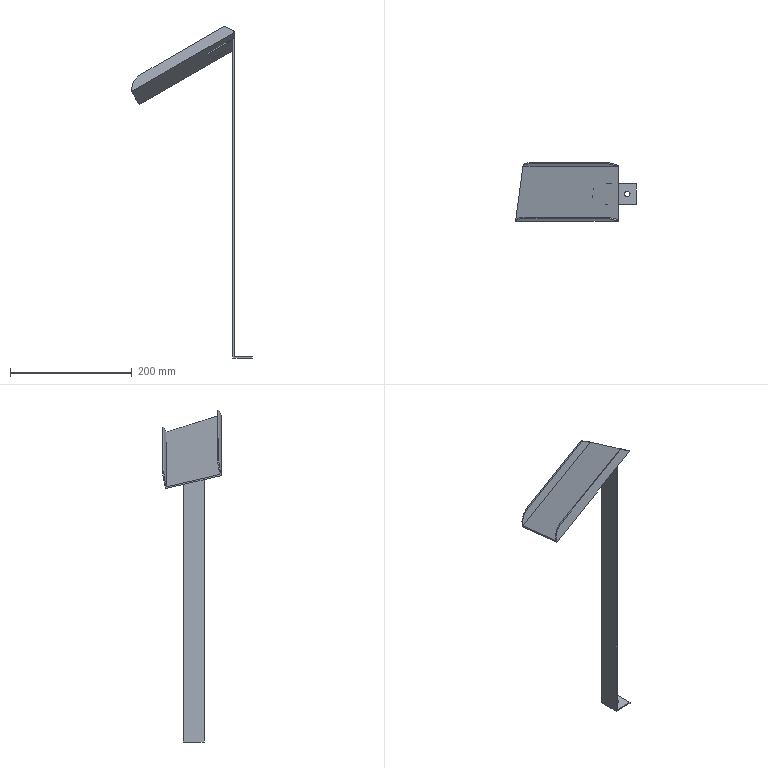Part | NX | features solid 2 | 1 solid | 27 faces | box 198.257 x 96.321 x 544.886 mm | volume 86995 mm3 | plane 24 | cylinder 3 | commonest cylinder face diameters 60 x2 9 x1
STEP:
#1=CARTESIAN_POINT('',(-340.,82.105,-151.35));
#2=VERTEX_POINT('',#1);
#3=CARTESIAN_POINT('',(-383.223,82.105,-176.304));
#4=VERTEX_POINT('',#3);
#5=CARTESIAN_POINT('',(-341.705,82.105,-152.334));
#6=DIRECTION('',(0.866,0.,0.5));
#7=VECTOR('',#6,1000.);
#8=LINE('',#5,#7);
#9=EDGE_CURVE('',#2,#4,#8,.F.);
#10=ORIENTED_EDGE('',*,*,#9,.F.);
#11=CARTESIAN_POINT('',(-340.,55.747,-143.195));
#12=VERTEX_POINT('',#11);
#13=CARTESIAN_POINT('',(-340.,-1199.843,245.286));
#14=DIRECTION('',(0.,0.9553,-0.2956));
#15=VECTOR('',#14,1000.);
#16=LINE('',#13,#15);
#17=EDGE_CURVE('',#12,#2,#16,.T.);
#18=ORIENTED_EDGE('',*,*,#17,.F.);
#19=CARTESIAN_POINT('',(-339.741,55.747,-143.045));
#20=VERTEX_POINT('',#19);
#21=CARTESIAN_POINT('',(-339.741,55.747,-143.045));
#22=DIRECTION('',(-0.866,0.,-0.5));
#23=VECTOR('',#22,1000.);
#24=LINE('',#21,#23);
#25=EDGE_CURVE('',#20,#12,#24,.T.);
#26=ORIENTED_EDGE('',*,*,#25,.F.);
#27=CARTESIAN_POINT('',(-340.,53.815,-142.597));
#28=VERTEX_POINT('',#27);
#29=CARTESIAN_POINT('',(-339.741,55.747,-143.045));
#30=DIRECTION('',(0.1294,0.9659,-0.2241));
#31=VECTOR('',#30,1000.);
#32=LINE('',#29,#31);
#33=EDGE_CURVE('',#20,#28,#32,.F.);
#34=ORIENTED_EDGE('',*,*,#33,.T.);
#35=CARTESIAN_POINT('',(-508.257,53.815,-239.74));
#36=VERTEX_POINT('',#35);
#37=CARTESIAN_POINT('',(-958.517,53.815,-499.698));
#38=DIRECTION('',(-0.866,0.,-0.5));
#39=VECTOR('',#38,1000.);
#40=LINE('',#37,#39);
#41=EDGE_CURVE('',#28,#36,#40,.T.);
#42=ORIENTED_EDGE('',*,*,#41,.T.);
#43=CARTESIAN_POINT('',(-495.958,145.615,-261.042));
#44=VERTEX_POINT('',#43);
#45=CARTESIAN_POINT('',(-693.776,-1330.922,81.59));
#46=DIRECTION('',(-0.1294,-0.9659,0.2241));
#47=VECTOR('',#46,1000.);
#48=LINE('',#45,#47);
#49=EDGE_CURVE('',#36,#44,#48,.F.);
#50=ORIENTED_EDGE('',*,*,#49,.T.);
#51=CARTESIAN_POINT('',(-340.,145.615,-171.));
#52=VERTEX_POINT('',#51);
#53=CARTESIAN_POINT('',(-946.218,145.615,-521.));
#54=DIRECTION('',(-0.866,0.,-0.5));
#55=VECTOR('',#54,1000.);
#56=LINE('',#53,#55);
#57=EDGE_CURVE('',#52,#44,#56,.T.);
#58=ORIENTED_EDGE('',*,*,#57,.F.);
#59=CARTESIAN_POINT('',(-340.,116.29,-161.927));
#60=VERTEX_POINT('',#59);
#61=CARTESIAN_POINT('',(-340.,-1199.843,245.286));
#62=DIRECTION('',(0.,0.9553,-0.2956));
#63=VECTOR('',#62,1000.);
#64=LINE('',#61,#63);
#65=EDGE_CURVE('',#60,#52,#64,.T.);
#66=ORIENTED_EDGE('',*,*,#65,.F.);
#67=CARTESIAN_POINT('',(-378.643,116.29,-184.237));
#68=VERTEX_POINT('',#67);
#69=CARTESIAN_POINT('',(-950.147,116.29,-514.195));
#70=DIRECTION('',(-0.866,0.,-0.5));
#71=VECTOR('',#70,1000.);
#72=LINE('',#69,#71);
#73=EDGE_CURVE('',#60,#68,#72,.T.);
#74=ORIENTED_EDGE('',*,*,#73,.T.);
#75=CARTESIAN_POINT('',(-572.533,-1330.922,151.59));
#76=DIRECTION('',(0.1294,0.9659,-0.2241));
#77=VECTOR('',#76,1000.);
#78=LINE('',#75,#77);
#79=EDGE_CURVE('',#4,#68,#78,.T.);
#80=ORIENTED_EDGE('',*,*,#79,.F.);
#81=EDGE_LOOP('',(#10,#18,#26,#34,#42,#50,#58,#66,#74,#80));
#82=FACE_BOUND('',#81,.T.);
#83=CARTESIAN_POINT('',(-1144.036,-1330.922,-178.368));
#84=DIRECTION('',(-0.483,0.2588,0.8365));
#85=DIRECTION('',(0.866,0.,0.5));
#86=AXIS2_PLACEMENT_3D('',#83,#84,#85);
#87=PLANE('',#86);
#88=ADVANCED_FACE('',(#82),#87,.F.);
#89=CARTESIAN_POINT('',(-340.,56.264,-140.964));
#90=VERTEX_POINT('',#89);
#91=CARTESIAN_POINT('',(-507.998,56.264,-237.957));
#92=VERTEX_POINT('',#91);
#93=CARTESIAN_POINT('',(-959.224,56.264,-498.473));
#94=DIRECTION('',(-0.866,0.,-0.5));
#95=VECTOR('',#94,1000.);
#96=LINE('',#93,#95);
#97=EDGE_CURVE('',#90,#92,#96,.T.);
#98=ORIENTED_EDGE('',*,*,#97,.F.);
#99=CARTESIAN_POINT('',(-340.,146.133,-168.769));
#100=VERTEX_POINT('',#99);
#101=CARTESIAN_POINT('',(-340.,-1199.168,247.468));
#102=DIRECTION('',(0.,0.9553,-0.2956));
#103=VECTOR('',#102,1000.);
#104=LINE('',#101,#103);
#105=EDGE_CURVE('',#90,#100,#104,.T.);
#106=ORIENTED_EDGE('',*,*,#105,.T.);
#107=CARTESIAN_POINT('',(-340.251,146.133,-168.914));
#108=VERTEX_POINT('',#107);
#109=CARTESIAN_POINT('',(-947.184,146.133,-519.327));
#110=DIRECTION('',(-0.866,0.,-0.5));
#111=VECTOR('',#110,1000.);
#112=LINE('',#109,#111);
#113=EDGE_CURVE('',#100,#108,#112,.T.);
#114=ORIENTED_EDGE('',*,*,#113,.T.);
#115=CARTESIAN_POINT('',(-340.51,144.201,-168.466));
#116=VERTEX_POINT('',#115);
#117=CARTESIAN_POINT('',(-538.07,-1330.404,173.717));
#118=DIRECTION('',(-0.1294,-0.9659,0.2241));
#119=VECTOR('',#118,1000.);
#120=LINE('',#117,#119);
#121=EDGE_CURVE('',#116,#108,#120,.F.);
#122=ORIENTED_EDGE('',*,*,#121,.F.);
#123=CARTESIAN_POINT('',(-496.216,144.201,-258.363));
#124=VERTEX_POINT('',#123);
#125=CARTESIAN_POINT('',(-947.443,144.201,-518.879));
#126=DIRECTION('',(-0.866,0.,-0.5));
#127=VECTOR('',#126,1000.);
#128=LINE('',#125,#127);
#129=EDGE_CURVE('',#116,#124,#128,.T.);
#130=ORIENTED_EDGE('',*,*,#129,.T.);
#131=CARTESIAN_POINT('',(-693.776,-1330.404,83.82));
#132=DIRECTION('',(-0.1294,-0.9659,0.2241));
#133=VECTOR('',#132,1000.);
#134=LINE('',#131,#133);
#135=EDGE_CURVE('',#92,#124,#134,.F.);
#136=ORIENTED_EDGE('',*,*,#135,.F.);
#137=EDGE_LOOP('',(#98,#106,#114,#122,#130,#136));
#138=FACE_BOUND('',#137,.T.);
#139=CARTESIAN_POINT('',(-1145.002,-1330.404,-176.695));
#140=DIRECTION('',(-0.483,0.2588,0.8365));
#141=DIRECTION('',(0.866,0.,0.5));
#142=AXIS2_PLACEMENT_3D('',#139,#140,#141);
#143=PLANE('',#142);
#144=ADVANCED_FACE('',(#138),#143,.T.);
#145=CARTESIAN_POINT('',(-340.,11.781,-332.662));
#146=DIRECTION('',(0.,0.226,0.9741));
#147=VECTOR('',#146,1000.);
#148=LINE('',#145,#147);
#149=EDGE_CURVE('',#12,#90,#148,.T.);
#150=ORIENTED_EDGE('',*,*,#149,.F.);
#151=ORIENTED_EDGE('',*,*,#17,.T.);
#152=CARTESIAN_POINT('',(-340.,82.105,-675.));
#153=VERTEX_POINT('',#152);
#154=CARTESIAN_POINT('',(-340.,82.105,-9.));
#155=DIRECTION('',(0.,0.,1.));
#156=VECTOR('',#155,1000.);
#157=LINE('',#154,#156);
#158=EDGE_CURVE('',#2,#153,#157,.F.);
#159=ORIENTED_EDGE('',*,*,#158,.T.);
#160=CARTESIAN_POINT('',(-340.,116.29,-675.));
#161=VERTEX_POINT('',#160);
#162=CARTESIAN_POINT('',(-340.,-710.,-675.));
#163=DIRECTION('',(0.,-1.,0.));
#164=VECTOR('',#163,1000.);
#165=LINE('',#162,#164);
#166=EDGE_CURVE('',#153,#161,#165,.F.);
#167=ORIENTED_EDGE('',*,*,#166,.T.);
#168=CARTESIAN_POINT('',(-340.,116.29,-163.531));
#169=VERTEX_POINT('',#168);
#170=CARTESIAN_POINT('',(-340.,116.29,-9.));
#171=DIRECTION('',(0.,0.,1.));
#172=VECTOR('',#171,1000.);
#173=LINE('',#170,#172);
#174=EDGE_CURVE('',#169,#161,#173,.F.);
#175=ORIENTED_EDGE('',*,*,#174,.F.);
#176=CARTESIAN_POINT('',(-340.,116.29,-9.));
#177=DIRECTION('',(0.,0.,1.));
#178=VECTOR('',#177,1000.);
#179=LINE('',#176,#178);
#180=EDGE_CURVE('',#60,#169,#179,.F.);
#181=ORIENTED_EDGE('',*,*,#180,.F.);
#182=ORIENTED_EDGE('',*,*,#65,.T.);
#183=CARTESIAN_POINT('',(-340.,103.18,-353.871));
#184=DIRECTION('',(0.,0.226,0.9741));
#185=VECTOR('',#184,1000.);
#186=LINE('',#183,#185);
#187=EDGE_CURVE('',#52,#100,#186,.T.);
#188=ORIENTED_EDGE('',*,*,#187,.T.);
#189=ORIENTED_EDGE('',*,*,#105,.F.);
#190=EDGE_LOOP('',(#150,#151,#159,#167,#175,#181,#182,#188,#189));
#191=FACE_BOUND('',#190,.T.);
#192=CARTESIAN_POINT('',(-340.,-1383.009,-9.));
#193=DIRECTION('',(1.,0.,0.));
#194=DIRECTION('',(0.,0.,-1.));
#195=AXIS2_PLACEMENT_3D('',#192,#193,#194);
#196=PLANE('',#195);
#197=ADVANCED_FACE('',(#191),#196,.T.);
#198=CARTESIAN_POINT('',(-340.251,54.333,-140.511));
#199=VERTEX_POINT('',#198);
#200=CARTESIAN_POINT('',(-340.,56.207,-140.946));
#201=VERTEX_POINT('',#200);
#202=CARTESIAN_POINT('',(-525.771,-1330.404,180.818));
#203=DIRECTION('',(-0.1294,-0.9659,0.2241));
#204=VECTOR('',#203,1000.);
#205=LINE('',#202,#204);
#206=EDGE_CURVE('',#199,#201,#205,.F.);
#207=ORIENTED_EDGE('',*,*,#206,.F.);
#208=CARTESIAN_POINT('',(-340.,54.333,-140.366));
#209=VERTEX_POINT('',#208);
#210=CARTESIAN_POINT('',(-959.483,54.333,-498.025));
#211=DIRECTION('',(-0.866,0.,-0.5));
#212=VECTOR('',#211,1000.);
#213=LINE('',#210,#212);
#214=EDGE_CURVE('',#209,#199,#213,.T.);
#215=ORIENTED_EDGE('',*,*,#214,.F.);
#216=CARTESIAN_POINT('',(-340.,-1199.168,247.468));
#217=DIRECTION('',(0.,0.9553,-0.2956));
#218=VECTOR('',#217,1000.);
#219=LINE('',#216,#218);
#220=EDGE_CURVE('',#209,#201,#219,.T.);
#221=ORIENTED_EDGE('',*,*,#220,.T.);
#222=EDGE_LOOP('',(#207,#215,#221));
#223=FACE_BOUND('',#222,.T.);
#224=CARTESIAN_POINT('',(-1145.002,-1330.404,-176.695));
#225=DIRECTION('',(-0.483,0.2588,0.8365));
#226=DIRECTION('',(0.866,0.,0.5));
#227=AXIS2_PLACEMENT_3D('',#224,#225,#226);
#228=PLANE('',#227);
#229=ADVANCED_FACE('',(#223),#228,.T.);
#230=CARTESIAN_POINT('',(-495.958,146.154,-258.723));
#231=VERTEX_POINT('',#230);
#232=CARTESIAN_POINT('',(-495.958,145.868,-259.956));
#233=DIRECTION('',(0.,-0.226,-0.9741));
#234=VECTOR('',#233,1000.);
#235=LINE('',#232,#234);
#236=EDGE_CURVE('',#44,#231,#235,.F.);
#237=ORIENTED_EDGE('',*,*,#236,.F.);
#238=ORIENTED_EDGE('',*,*,#49,.F.);
#239=CARTESIAN_POINT('',(-508.257,54.353,-237.421));
#240=VERTEX_POINT('',#239);
#241=CARTESIAN_POINT('',(-508.257,54.067,-238.653));
#242=DIRECTION('',(0.,-0.226,-0.9741));
#243=VECTOR('',#242,1000.);
#244=LINE('',#241,#243);
#245=EDGE_CURVE('',#36,#240,#244,.F.);
#246=ORIENTED_EDGE('',*,*,#245,.T.);
#247=CARTESIAN_POINT('',(-507.998,56.285,-237.869));
#248=VERTEX_POINT('',#247);
#249=CARTESIAN_POINT('',(-495.958,146.154,-258.723));
#250=DIRECTION('',(-0.1294,-0.9659,0.2241));
#251=VECTOR('',#250,1000.);
#252=LINE('',#249,#251);
#253=EDGE_CURVE('',#240,#248,#252,.F.);
#254=ORIENTED_EDGE('',*,*,#253,.T.);
#255=CARTESIAN_POINT('',(-507.998,55.999,-239.102));
#256=DIRECTION('',(0.,-0.226,-0.9741));
#257=VECTOR('',#256,1000.);
#258=LINE('',#255,#257);
#259=EDGE_CURVE('',#92,#248,#258,.F.);
#260=ORIENTED_EDGE('',*,*,#259,.F.);
#261=ORIENTED_EDGE('',*,*,#135,.T.);
#262=CARTESIAN_POINT('',(-496.216,144.222,-258.275));
#263=VERTEX_POINT('',#262);
#264=CARTESIAN_POINT('',(-496.216,143.936,-259.507));
#265=DIRECTION('',(0.,-0.226,-0.9741));
#266=VECTOR('',#265,1000.);
#267=LINE('',#264,#266);
#268=EDGE_CURVE('',#124,#263,#267,.F.);
#269=ORIENTED_EDGE('',*,*,#268,.T.);
#270=CARTESIAN_POINT('',(-495.958,146.154,-258.723));
#271=DIRECTION('',(0.1294,0.9659,-0.2241));
#272=VECTOR('',#271,1000.);
#273=LINE('',#270,#272);
#274=EDGE_CURVE('',#263,#231,#273,.T.);
#275=ORIENTED_EDGE('',*,*,#274,.T.);
#276=EDGE_LOOP('',(#237,#238,#246,#254,#260,#261,#269,#275));
#277=FACE_BOUND('',#276,.T.);
#278=CARTESIAN_POINT('',(-495.958,145.868,-259.956));
#279=DIRECTION('',(-0.9916,0.1261,-0.02925));
#280=DIRECTION('',(0.,0.226,0.9741));
#281=AXIS2_PLACEMENT_3D('',#278,#279,#280);
#282=PLANE('',#281);
#283=ADVANCED_FACE('',(#277),#282,.T.);
#284=ORIENTED_EDGE('',*,*,#113,.F.);
#285=ORIENTED_EDGE('',*,*,#187,.F.);
#286=ORIENTED_EDGE('',*,*,#57,.T.);
#287=ORIENTED_EDGE('',*,*,#236,.T.);
#288=CARTESIAN_POINT('',(-480.699,150.136,-232.75));
#289=VERTEX_POINT('',#288);
#290=CARTESIAN_POINT('',(-466.21,142.372,-257.846));
#291=DIRECTION('',(0.1294,0.9659,-0.2241));
#292=DIRECTION('',(0.,0.226,0.9741));
#293=AXIS2_PLACEMENT_3D('',#290,#291,#292);
#294=CIRCLE('',#293,30.);
#295=EDGE_CURVE('',#231,#289,#294,.T.);
#296=ORIENTED_EDGE('',*,*,#295,.T.);
#297=CARTESIAN_POINT('',(-355.588,150.136,-160.518));
#298=VERTEX_POINT('',#297);
#299=CARTESIAN_POINT('',(-340.,150.136,-151.518));
#300=DIRECTION('',(-0.866,0.,-0.5));
#301=VECTOR('',#300,1000.);
#302=LINE('',#299,#301);
#303=EDGE_CURVE('',#298,#289,#302,.T.);
#304=ORIENTED_EDGE('',*,*,#303,.F.);
#305=CARTESIAN_POINT('',(-339.134,145.841,-169.526));
#306=DIRECTION('',(-0.855,0.2232,0.4681));
#307=VECTOR('',#306,1000.);
#308=LINE('',#305,#307);
#309=EDGE_CURVE('',#298,#108,#308,.F.);
#310=ORIENTED_EDGE('',*,*,#309,.T.);
#311=EDGE_LOOP('',(#284,#285,#286,#287,#296,#304,#310));
#312=FACE_BOUND('',#311,.T.);
#313=CARTESIAN_POINT('',(-340.,145.615,-171.));
#314=DIRECTION('',(0.1294,0.9659,-0.2241));
#315=DIRECTION('',(-0.866,0.,-0.5));
#316=AXIS2_PLACEMENT_3D('',#313,#314,#315);
#317=PLANE('',#316);
#318=ADVANCED_FACE('',(#312),#317,.T.);
#319=CARTESIAN_POINT('',(-340.,54.267,-140.649));
#320=VERTEX_POINT('',#319);
#321=CARTESIAN_POINT('',(-340.,-1369.713,77.708));
#322=DIRECTION('',(0.,0.9884,-0.1516));
#323=VECTOR('',#322,1000.);
#324=LINE('',#321,#323);
#325=EDGE_CURVE('',#201,#320,#324,.F.);
#326=ORIENTED_EDGE('',*,*,#325,.F.);
#327=ORIENTED_EDGE('',*,*,#220,.F.);
#328=CARTESIAN_POINT('',(-340.,9.816,-332.206));
#329=DIRECTION('',(0.,0.226,0.9741));
#330=VECTOR('',#329,1000.);
#331=LINE('',#328,#330);
#332=EDGE_CURVE('',#320,#209,#331,.T.);
#333=ORIENTED_EDGE('',*,*,#332,.F.);
#334=EDGE_LOOP('',(#326,#327,#333));
#335=FACE_BOUND('',#334,.T.);
#336=CARTESIAN_POINT('',(-340.,-1383.009,-9.));
#337=DIRECTION('',(1.,0.,0.));
#338=DIRECTION('',(0.,0.,-1.));
#339=AXIS2_PLACEMENT_3D('',#336,#337,#338);
#340=PLANE('',#339);
#341=ADVANCED_FACE('',(#335),#340,.T.);
#342=ORIENTED_EDGE('',*,*,#214,.T.);
#343=CARTESIAN_POINT('',(-355.588,58.336,-132.114));
#344=VERTEX_POINT('',#343);
#345=CARTESIAN_POINT('',(-340.,54.267,-140.649));
#346=DIRECTION('',(0.855,-0.2232,-0.4681));
#347=VECTOR('',#346,1000.);
#348=LINE('',#345,#347);
#349=EDGE_CURVE('',#199,#344,#348,.F.);
#350=ORIENTED_EDGE('',*,*,#349,.T.);
#351=CARTESIAN_POINT('',(-492.998,58.336,-211.448));
#352=VERTEX_POINT('',#351);
#353=CARTESIAN_POINT('',(-340.,58.336,-123.114));
#354=DIRECTION('',(-0.866,0.,-0.5));
#355=VECTOR('',#354,1000.);
#356=LINE('',#353,#355);
#357=EDGE_CURVE('',#344,#352,#356,.T.);
#358=ORIENTED_EDGE('',*,*,#357,.T.);
#359=CARTESIAN_POINT('',(-478.509,50.571,-236.543));
#360=DIRECTION('',(0.1294,0.9659,-0.2241));
#361=DIRECTION('',(0.,0.226,0.9741));
#362=AXIS2_PLACEMENT_3D('',#359,#360,#361);
#363=CIRCLE('',#362,30.);
#364=EDGE_CURVE('',#352,#240,#363,.F.);
#365=ORIENTED_EDGE('',*,*,#364,.T.);
#366=ORIENTED_EDGE('',*,*,#245,.F.);
#367=ORIENTED_EDGE('',*,*,#41,.F.);
#368=CARTESIAN_POINT('',(-340.,9.816,-332.206));
#369=DIRECTION('',(0.,0.226,0.9741));
#370=VECTOR('',#369,1000.);
#371=LINE('',#368,#370);
#372=EDGE_CURVE('',#28,#320,#371,.T.);
#373=ORIENTED_EDGE('',*,*,#372,.T.);
#374=ORIENTED_EDGE('',*,*,#332,.T.);
#375=EDGE_LOOP('',(#342,#350,#358,#365,#366,#367,#373,#374));
#376=FACE_BOUND('',#375,.T.);
#377=CARTESIAN_POINT('',(-352.299,53.815,-149.698));
#378=DIRECTION('',(0.1294,0.9659,-0.2241));
#379=DIRECTION('',(-0.866,0.,-0.5));
#380=AXIS2_PLACEMENT_3D('',#377,#378,#379);
#381=PLANE('',#380);
#382=ADVANCED_FACE('',(#376),#381,.F.);
#383=CARTESIAN_POINT('',(-355.847,148.204,-160.069));
#384=VERTEX_POINT('',#383);
#385=CARTESIAN_POINT('',(-480.958,148.204,-232.302));
#386=VERTEX_POINT('',#385);
#387=CARTESIAN_POINT('',(-340.259,148.204,-151.069));
#388=DIRECTION('',(-0.866,0.,-0.5));
#389=VECTOR('',#388,1000.);
#390=LINE('',#387,#389);
#391=EDGE_CURVE('',#384,#386,#390,.T.);
#392=ORIENTED_EDGE('',*,*,#391,.F.);
#393=CARTESIAN_POINT('',(-355.588,150.136,-160.518));
#394=DIRECTION('',(0.1294,0.9659,-0.2241));
#395=VECTOR('',#394,1000.);
#396=LINE('',#393,#395);
#397=EDGE_CURVE('',#384,#298,#396,.T.);
#398=ORIENTED_EDGE('',*,*,#397,.T.);
#399=ORIENTED_EDGE('',*,*,#303,.T.);
#400=CARTESIAN_POINT('',(-480.699,150.136,-232.75));
#401=DIRECTION('',(-0.1294,-0.9659,0.2241));
#402=VECTOR('',#401,1000.);
#403=LINE('',#400,#402);
#404=EDGE_CURVE('',#289,#386,#403,.T.);
#405=ORIENTED_EDGE('',*,*,#404,.T.);
#406=EDGE_LOOP('',(#392,#398,#399,#405));
#407=FACE_BOUND('',#406,.T.);
#408=CARTESIAN_POINT('',(-340.,150.136,-151.518));
#409=DIRECTION('',(0.483,-0.2588,-0.8365));
#410=DIRECTION('',(-0.866,0.,-0.5));
#411=AXIS2_PLACEMENT_3D('',#408,#409,#410);
#412=PLANE('',#411);
#413=ADVANCED_FACE('',(#407),#412,.F.);
#414=ORIENTED_EDGE('',*,*,#129,.F.);
#415=CARTESIAN_POINT('',(-340.259,144.136,-168.603));
#416=DIRECTION('',(0.855,-0.2232,-0.4681));
#417=VECTOR('',#416,1000.);
#418=LINE('',#415,#417);
#419=EDGE_CURVE('',#116,#384,#418,.F.);
#420=ORIENTED_EDGE('',*,*,#419,.T.);
#421=ORIENTED_EDGE('',*,*,#391,.T.);
#422=CARTESIAN_POINT('',(-466.469,140.44,-257.397));
#423=DIRECTION('',(0.1294,0.9659,-0.2241));
#424=DIRECTION('',(0.,0.226,0.9741));
#425=AXIS2_PLACEMENT_3D('',#422,#423,#424);
#426=CIRCLE('',#425,30.);
#427=EDGE_CURVE('',#386,#263,#426,.F.);
#428=ORIENTED_EDGE('',*,*,#427,.T.);
#429=ORIENTED_EDGE('',*,*,#268,.F.);
#430=EDGE_LOOP('',(#414,#420,#421,#428,#429));
#431=FACE_BOUND('',#430,.T.);
#432=CARTESIAN_POINT('',(-340.259,143.684,-170.552));
#433=DIRECTION('',(0.1294,0.9659,-0.2241));
#434=DIRECTION('',(0.,0.226,0.9741));
#435=AXIS2_PLACEMENT_3D('',#432,#433,#434);
#436=PLANE('',#435);
#437=ADVANCED_FACE('',(#431),#436,.F.);
#438=ORIENTED_EDGE('',*,*,#295,.F.);
#439=ORIENTED_EDGE('',*,*,#274,.F.);
#440=ORIENTED_EDGE('',*,*,#427,.F.);
#441=ORIENTED_EDGE('',*,*,#404,.F.);
#442=EDGE_LOOP('',(#438,#439,#440,#441));
#443=FACE_BOUND('',#442,.T.);
#444=CARTESIAN_POINT('',(-466.21,142.372,-257.846));
#445=DIRECTION('',(-0.1294,-0.9659,0.2241));
#446=DIRECTION('',(0.,-0.226,-0.9741));
#447=AXIS2_PLACEMENT_3D('',#444,#445,#446);
#448=CYLINDRICAL_SURFACE('',#447,30.);
#449=ADVANCED_FACE('',(#443),#448,.T.);
#450=ORIENTED_EDGE('',*,*,#419,.F.);
#451=ORIENTED_EDGE('',*,*,#121,.T.);
#452=ORIENTED_EDGE('',*,*,#309,.F.);
#453=ORIENTED_EDGE('',*,*,#397,.F.);
#454=EDGE_LOOP('',(#450,#451,#452,#453));
#455=FACE_BOUND('',#454,.T.);
#456=CARTESIAN_POINT('',(-340.,146.068,-169.052));
#457=DIRECTION('',(-0.5022,-0.1311,-0.8548));
#458=DIRECTION('',(-0.8622,0.,0.5065));
#459=AXIS2_PLACEMENT_3D('',#456,#457,#458);
#460=PLANE('',#459);
#461=ADVANCED_FACE('',(#455),#460,.F.);
#462=ORIENTED_EDGE('',*,*,#357,.F.);
#463=CARTESIAN_POINT('',(-355.33,60.268,-132.563));
#464=VERTEX_POINT('',#463);
#465=CARTESIAN_POINT('',(-355.33,60.268,-132.563));
#466=DIRECTION('',(0.1294,0.9659,-0.2241));
#467=VECTOR('',#466,1000.);
#468=LINE('',#465,#467);
#469=EDGE_CURVE('',#344,#464,#468,.T.);
#470=ORIENTED_EDGE('',*,*,#469,.T.);
#471=CARTESIAN_POINT('',(-492.739,60.268,-211.896));
#472=VERTEX_POINT('',#471);
#473=CARTESIAN_POINT('',(-339.741,60.268,-123.563));
#474=DIRECTION('',(-0.866,0.,-0.5));
#475=VECTOR('',#474,1000.);
#476=LINE('',#473,#475);
#477=EDGE_CURVE('',#464,#472,#476,.T.);
#478=ORIENTED_EDGE('',*,*,#477,.T.);
#479=CARTESIAN_POINT('',(-492.739,60.268,-211.896));
#480=DIRECTION('',(0.1294,0.9659,-0.2241));
#481=VECTOR('',#480,1000.);
#482=LINE('',#479,#481);
#483=EDGE_CURVE('',#472,#352,#482,.F.);
#484=ORIENTED_EDGE('',*,*,#483,.T.);
#485=EDGE_LOOP('',(#462,#470,#478,#484));
#486=FACE_BOUND('',#485,.T.);
#487=CARTESIAN_POINT('',(-339.741,60.268,-123.563));
#488=DIRECTION('',(0.483,-0.2588,-0.8365));
#489=DIRECTION('',(-0.866,0.,-0.5));
#490=AXIS2_PLACEMENT_3D('',#487,#488,#489);
#491=PLANE('',#490);
#492=ADVANCED_FACE('',(#486),#491,.F.);
#493=CARTESIAN_POINT('',(-339.741,56.199,-141.097));
#494=VERTEX_POINT('',#493);
#495=CARTESIAN_POINT('',(-339.741,55.747,-143.045));
#496=DIRECTION('',(0.,0.226,0.9741));
#497=VECTOR('',#496,1000.);
#498=LINE('',#495,#497);
#499=EDGE_CURVE('',#20,#494,#498,.T.);
#500=ORIENTED_EDGE('',*,*,#499,.T.);
#501=CARTESIAN_POINT('',(-339.741,56.199,-141.097));
#502=DIRECTION('',(-0.1294,-0.9659,0.2241));
#503=VECTOR('',#502,1000.);
#504=LINE('',#501,#503);
#505=EDGE_CURVE('',#494,#320,#504,.T.);
#506=ORIENTED_EDGE('',*,*,#505,.T.);
#507=ORIENTED_EDGE('',*,*,#372,.F.);
#508=ORIENTED_EDGE('',*,*,#33,.F.);
#509=EDGE_LOOP('',(#500,#506,#507,#508));
#510=FACE_BOUND('',#509,.T.);
#511=CARTESIAN_POINT('',(-339.741,55.747,-143.045));
#512=DIRECTION('',(-0.9916,0.1261,-0.02925));
#513=DIRECTION('',(0.,0.226,0.9741));
#514=AXIS2_PLACEMENT_3D('',#511,#512,#513);
#515=PLANE('',#514);
#516=ADVANCED_FACE('',(#510),#515,.F.);
#517=ORIENTED_EDGE('',*,*,#149,.T.);
#518=ORIENTED_EDGE('',*,*,#97,.T.);
#519=ORIENTED_EDGE('',*,*,#259,.T.);
#520=CARTESIAN_POINT('',(-478.25,52.503,-236.992));
#521=DIRECTION('',(0.1294,0.9659,-0.2241));
#522=DIRECTION('',(0.,0.226,0.9741));
#523=AXIS2_PLACEMENT_3D('',#520,#521,#522);
#524=CIRCLE('',#523,30.);
#525=EDGE_CURVE('',#248,#472,#524,.T.);
#526=ORIENTED_EDGE('',*,*,#525,.T.);
#527=ORIENTED_EDGE('',*,*,#477,.F.);
#528=CARTESIAN_POINT('',(-338.875,55.973,-141.571));
#529=DIRECTION('',(-0.855,0.2232,0.4681));
#530=VECTOR('',#529,1000.);
#531=LINE('',#528,#530);
#532=EDGE_CURVE('',#464,#494,#531,.F.);
#533=ORIENTED_EDGE('',*,*,#532,.T.);
#534=ORIENTED_EDGE('',*,*,#499,.F.);
#535=ORIENTED_EDGE('',*,*,#25,.T.);
#536=EDGE_LOOP('',(#517,#518,#519,#526,#527,#533,#534,#535));
#537=FACE_BOUND('',#536,.T.);
#538=CARTESIAN_POINT('',(-339.741,55.747,-143.045));
#539=DIRECTION('',(0.1294,0.9659,-0.2241));
#540=DIRECTION('',(0.,0.226,0.9741));
#541=AXIS2_PLACEMENT_3D('',#538,#539,#540);
#542=PLANE('',#541);
#543=ADVANCED_FACE('',(#537),#542,.T.);
#544=ORIENTED_EDGE('',*,*,#525,.F.);
#545=ORIENTED_EDGE('',*,*,#253,.F.);
#546=ORIENTED_EDGE('',*,*,#364,.F.);
#547=ORIENTED_EDGE('',*,*,#483,.F.);
#548=EDGE_LOOP('',(#544,#545,#546,#547));
#549=FACE_BOUND('',#548,.T.);
#550=CARTESIAN_POINT('',(-478.25,52.503,-236.992));
#551=DIRECTION('',(0.1294,0.9659,-0.2241));
#552=DIRECTION('',(0.,0.226,0.9741));
#553=AXIS2_PLACEMENT_3D('',#550,#551,#552);
#554=CYLINDRICAL_SURFACE('',#553,30.);
#555=ADVANCED_FACE('',(#549),#554,.T.);
#556=ORIENTED_EDGE('',*,*,#349,.F.);
#557=ORIENTED_EDGE('',*,*,#206,.T.);
#558=ORIENTED_EDGE('',*,*,#325,.T.);
#559=ORIENTED_EDGE('',*,*,#505,.F.);
#560=ORIENTED_EDGE('',*,*,#532,.F.);
#561=ORIENTED_EDGE('',*,*,#469,.F.);
#562=EDGE_LOOP('',(#556,#557,#558,#559,#560,#561));
#563=FACE_BOUND('',#562,.T.);
#564=CARTESIAN_POINT('',(-339.741,56.199,-141.097));
#565=DIRECTION('',(-0.5022,-0.1311,-0.8548));
#566=DIRECTION('',(-0.8622,0.,0.5065));
#567=AXIS2_PLACEMENT_3D('',#564,#565,#566);
#568=PLANE('',#567);
#569=ADVANCED_FACE('',(#563),#568,.F.);
#570=ORIENTED_EDGE('',*,*,#79,.T.);
#571=CARTESIAN_POINT('',(-377.608,116.29,-186.03));
#572=VERTEX_POINT('',#571);
#573=CARTESIAN_POINT('',(-571.567,116.29,149.916));
#574=DIRECTION('',(-0.5,0.,0.866));
#575=VECTOR('',#574,1000.);
#576=LINE('',#573,#575);
#577=EDGE_CURVE('',#572,#68,#576,.T.);
#578=ORIENTED_EDGE('',*,*,#577,.F.);
#579=CARTESIAN_POINT('',(-382.188,82.105,-178.098));
#580=VERTEX_POINT('',#579);
#581=CARTESIAN_POINT('',(-571.567,-1331.44,149.916));
#582=DIRECTION('',(0.1294,0.9659,-0.2241));
#583=VECTOR('',#582,1000.);
#584=LINE('',#581,#583);
#585=EDGE_CURVE('',#580,#572,#584,.T.);
#586=ORIENTED_EDGE('',*,*,#585,.F.);
#587=CARTESIAN_POINT('',(-571.567,82.105,149.916));
#588=DIRECTION('',(-0.5,0.,0.866));
#589=VECTOR('',#588,1000.);
#590=LINE('',#587,#589);
#591=EDGE_CURVE('',#580,#4,#590,.T.);
#592=ORIENTED_EDGE('',*,*,#591,.T.);
#593=EDGE_LOOP('',(#570,#578,#586,#592));
#594=FACE_BOUND('',#593,.T.);
#595=CARTESIAN_POINT('',(-571.567,-1331.44,149.916));
#596=DIRECTION('',(0.866,0.,0.5));
#597=DIRECTION('',(0.5,0.,-0.866));
#598=AXIS2_PLACEMENT_3D('',#595,#596,#597);
#599=PLANE('',#598);
#600=ADVANCED_FACE('',(#594),#599,.F.);
#601=ORIENTED_EDGE('',*,*,#73,.F.);
#602=ORIENTED_EDGE('',*,*,#180,.T.);
#603=CARTESIAN_POINT('',(-342.,116.29,-164.685));
#604=VERTEX_POINT('',#603);
#605=CARTESIAN_POINT('',(-949.452,116.29,-515.398));
#606=DIRECTION('',(0.866,0.,0.5));
#607=VECTOR('',#606,1000.);
#608=LINE('',#605,#607);
#609=EDGE_CURVE('',#169,#604,#608,.F.);
#610=ORIENTED_EDGE('',*,*,#609,.T.);
#611=ORIENTED_EDGE('',*,*,#609,.F.);
#612=ORIENTED_EDGE('',*,*,#174,.T.);
#613=CARTESIAN_POINT('',(-310.,116.29,-675.));
#614=VERTEX_POINT('',#613);
#615=CARTESIAN_POINT('',(-340.,116.29,-675.));
#616=DIRECTION('',(-1.,0.,0.));
#617=VECTOR('',#616,1000.);
#618=LINE('',#615,#617);
#619=EDGE_CURVE('',#614,#161,#618,.T.);
#620=ORIENTED_EDGE('',*,*,#619,.F.);
#621=CARTESIAN_POINT('',(-310.,116.29,-677.));
#622=VERTEX_POINT('',#621);
#623=CARTESIAN_POINT('',(-310.,116.29,-162.771));
#624=DIRECTION('',(0.,0.,-1.));
#625=VECTOR('',#624,1000.);
#626=LINE('',#623,#625);
#627=EDGE_CURVE('',#622,#614,#626,.F.);
#628=ORIENTED_EDGE('',*,*,#627,.F.);
#629=CARTESIAN_POINT('',(-342.,116.29,-677.));
#630=VERTEX_POINT('',#629);
#631=CARTESIAN_POINT('',(-340.,116.29,-677.));
#632=DIRECTION('',(-1.,0.,0.));
#633=VECTOR('',#632,1000.);
#634=LINE('',#631,#633);
#635=EDGE_CURVE('',#622,#630,#634,.T.);
#636=ORIENTED_EDGE('',*,*,#635,.T.);
#637=CARTESIAN_POINT('',(-342.,116.29,-165.472));
#638=VERTEX_POINT('',#637);
#639=CARTESIAN_POINT('',(-342.,116.29,-162.771));
#640=DIRECTION('',(0.,0.,1.));
#641=VECTOR('',#640,1000.);
#642=LINE('',#639,#641);
#643=EDGE_CURVE('',#638,#630,#642,.F.);
#644=ORIENTED_EDGE('',*,*,#643,.F.);
#645=CARTESIAN_POINT('',(-949.111,116.29,-515.988));
#646=DIRECTION('',(-0.866,0.,-0.5));
#647=VECTOR('',#646,1000.);
#648=LINE('',#645,#647);
#649=EDGE_CURVE('',#638,#572,#648,.T.);
#650=ORIENTED_EDGE('',*,*,#649,.T.);
#651=ORIENTED_EDGE('',*,*,#577,.T.);
#652=EDGE_LOOP('',(#601,#602,#610,#611,#612,#620,#628,#636,#644,#650,#651));
#653=FACE_BOUND('',#652,.T.);
#654=CARTESIAN_POINT('',(-340.,116.29,-162.771));
#655=DIRECTION('',(0.,1.,0.));
#656=DIRECTION('',(0.,0.,-1.));
#657=AXIS2_PLACEMENT_3D('',#654,#655,#656);
#658=PLANE('',#657);
#659=ADVANCED_FACE('',(#653),#658,.T.);
#660=ORIENTED_EDGE('',*,*,#649,.F.);
#661=CARTESIAN_POINT('',(-342.,87.105,-156.442));
#662=VERTEX_POINT('',#661);
#663=CARTESIAN_POINT('',(-342.,-1200.844,242.05));
#664=DIRECTION('',(0.,-0.9553,0.2956));
#665=VECTOR('',#664,1000.);
#666=LINE('',#663,#665);
#667=EDGE_CURVE('',#638,#662,#666,.T.);
#668=ORIENTED_EDGE('',*,*,#667,.T.);
#669=CARTESIAN_POINT('',(-342.,82.105,-154.895));
#670=VERTEX_POINT('',#669);
#671=CARTESIAN_POINT('',(-342.,86.779,-156.341));
#672=DIRECTION('',(0.,0.9553,-0.2956));
#673=VECTOR('',#672,1000.);
#674=LINE('',#671,#673);
#675=EDGE_CURVE('',#670,#662,#674,.T.);
#676=ORIENTED_EDGE('',*,*,#675,.F.);
#677=CARTESIAN_POINT('',(-953.691,82.105,-508.055));
#678=DIRECTION('',(-0.866,0.,-0.5));
#679=VECTOR('',#678,1000.);
#680=LINE('',#677,#679);
#681=EDGE_CURVE('',#670,#580,#680,.T.);
#682=ORIENTED_EDGE('',*,*,#681,.T.);
#683=ORIENTED_EDGE('',*,*,#585,.T.);
#684=EDGE_LOOP('',(#660,#668,#676,#682,#683));
#685=FACE_BOUND('',#684,.T.);
#686=CARTESIAN_POINT('',(-1143.07,-1331.44,-180.041));
#687=DIRECTION('',(-0.483,0.2588,0.8365));
#688=DIRECTION('',(0.866,0.,0.5));
#689=AXIS2_PLACEMENT_3D('',#686,#687,#688);
#690=PLANE('',#689);
#691=ADVANCED_FACE('',(#685),#690,.F.);
#692=CARTESIAN_POINT('',(-310.,82.105,-675.));
#693=VERTEX_POINT('',#692);
#694=CARTESIAN_POINT('',(-765.,82.105,-675.));
#695=DIRECTION('',(1.,0.,0.));
#696=VECTOR('',#695,1000.);
#697=LINE('',#694,#696);
#698=EDGE_CURVE('',#693,#153,#697,.F.);
#699=ORIENTED_EDGE('',*,*,#698,.T.);
#700=ORIENTED_EDGE('',*,*,#158,.F.);
#701=ORIENTED_EDGE('',*,*,#9,.T.);
#702=ORIENTED_EDGE('',*,*,#591,.F.);
#703=ORIENTED_EDGE('',*,*,#681,.F.);
#704=CARTESIAN_POINT('',(-342.,82.105,-156.442));
#705=VERTEX_POINT('',#704);
#706=CARTESIAN_POINT('',(-342.,82.105,-155.288));
#707=DIRECTION('',(0.,0.,-1.));
#708=VECTOR('',#707,1000.);
#709=LINE('',#706,#708);
#710=EDGE_CURVE('',#670,#705,#709,.T.);
#711=ORIENTED_EDGE('',*,*,#710,.T.);
#712=CARTESIAN_POINT('',(-342.,82.105,-677.));
#713=VERTEX_POINT('',#712);
#714=CARTESIAN_POINT('',(-342.,82.105,-155.288));
#715=DIRECTION('',(0.,0.,-1.));
#716=VECTOR('',#715,1000.);
#717=LINE('',#714,#716);
#718=EDGE_CURVE('',#705,#713,#717,.T.);
#719=ORIENTED_EDGE('',*,*,#718,.T.);
#720=CARTESIAN_POINT('',(-310.,82.105,-677.));
#721=VERTEX_POINT('',#720);
#722=CARTESIAN_POINT('',(-765.,82.105,-677.));
#723=DIRECTION('',(1.,0.,0.));
#724=VECTOR('',#723,1000.);
#725=LINE('',#722,#724);
#726=EDGE_CURVE('',#721,#713,#725,.F.);
#727=ORIENTED_EDGE('',*,*,#726,.F.);
#728=CARTESIAN_POINT('',(-310.,82.105,0.));
#729=DIRECTION('',(0.,0.,1.));
#730=VECTOR('',#729,1000.);
#731=LINE('',#728,#730);
#732=EDGE_CURVE('',#721,#693,#731,.T.);
#733=ORIENTED_EDGE('',*,*,#732,.T.);
#734=EDGE_LOOP('',(#699,#700,#701,#702,#703,#711,#719,#727,#733));
#735=FACE_BOUND('',#734,.T.);
#736=CARTESIAN_POINT('',(-340.,82.105,-155.288));
#737=DIRECTION('',(0.,1.,0.));
#738=DIRECTION('',(0.,0.,-1.));
#739=AXIS2_PLACEMENT_3D('',#736,#737,#738);
#740=PLANE('',#739);
#741=ADVANCED_FACE('',(#735),#740,.F.);
#742=ORIENTED_EDGE('',*,*,#710,.F.);
#743=ORIENTED_EDGE('',*,*,#675,.T.);
#744=CARTESIAN_POINT('',(-342.,87.105,-156.442));
#745=CARTESIAN_POINT('',(-342.,85.438,-156.442));
#746=CARTESIAN_POINT('',(-342.,83.771,-156.442));
#747=CARTESIAN_POINT('',(-342.,82.105,-156.442));
#748=B_SPLINE_CURVE_WITH_KNOTS('',3,(#744,#745,#746,#747),.UNSPECIFIED.,.F.,.F.,(4,4),(0.,1.),.UNSPECIFIED.);
#749=EDGE_CURVE('',#662,#705,#748,.T.);
#750=ORIENTED_EDGE('',*,*,#749,.T.);
#751=EDGE_LOOP('',(#742,#743,#750));
#752=FACE_BOUND('',#751,.T.);
#753=CARTESIAN_POINT('',(-342.,87.105,-155.288));
#754=DIRECTION('',(-1.,0.,0.));
#755=DIRECTION('',(0.,0.,1.));
#756=AXIS2_PLACEMENT_3D('',#753,#754,#755);
#757=PLANE('',#756);
#758=ADVANCED_FACE('',(#752),#757,.T.);
#759=ORIENTED_EDGE('',*,*,#667,.F.);
#760=ORIENTED_EDGE('',*,*,#643,.T.);
#761=CARTESIAN_POINT('',(-342.,87.105,-677.));
#762=DIRECTION('',(0.,-1.,0.));
#763=VECTOR('',#762,1000.);
#764=LINE('',#761,#763);
#765=EDGE_CURVE('',#713,#630,#764,.F.);
#766=ORIENTED_EDGE('',*,*,#765,.F.);
#767=ORIENTED_EDGE('',*,*,#718,.F.);
#768=ORIENTED_EDGE('',*,*,#749,.F.);
#769=EDGE_LOOP('',(#759,#760,#766,#767,#768));
#770=FACE_BOUND('',#769,.T.);
#771=CARTESIAN_POINT('',(-342.,87.105,-155.288));
#772=DIRECTION('',(-1.,0.,0.));
#773=DIRECTION('',(0.,0.,1.));
#774=AXIS2_PLACEMENT_3D('',#771,#772,#773);
#775=PLANE('',#774);
#776=ADVANCED_FACE('',(#770),#775,.T.);
#777=CARTESIAN_POINT('',(-329.5,99.7,-675.));
#778=VERTEX_POINT('',#777);
#779=CARTESIAN_POINT('',(-325.,99.7,-675.));
#780=DIRECTION('',(0.,0.,-1.));
#781=DIRECTION('',(-1.,0.,0.));
#782=AXIS2_PLACEMENT_3D('',#779,#780,#781);
#783=CIRCLE('',#782,4.5);
#784=EDGE_CURVE('',#778,#778,#783,.F.);
#785=ORIENTED_EDGE('',*,*,#784,.F.);
#786=EDGE_LOOP('',(#785));
#787=FACE_BOUND('',#786,.T.);
#788=ORIENTED_EDGE('',*,*,#166,.F.);
#789=ORIENTED_EDGE('',*,*,#698,.F.);
#790=CARTESIAN_POINT('',(-310.,-710.,-675.));
#791=DIRECTION('',(0.,-1.,0.));
#792=VECTOR('',#791,1000.);
#793=LINE('',#790,#792);
#794=EDGE_CURVE('',#693,#614,#793,.F.);
#795=ORIENTED_EDGE('',*,*,#794,.T.);
#796=ORIENTED_EDGE('',*,*,#619,.T.);
#797=EDGE_LOOP('',(#788,#789,#795,#796));
#798=FACE_BOUND('',#797,.T.);
#799=CARTESIAN_POINT('',(-765.,-710.,-675.));
#800=DIRECTION('',(0.,0.,-1.));
#801=DIRECTION('',(1.,0.,0.));
#802=AXIS2_PLACEMENT_3D('',#799,#800,#801);
#803=PLANE('',#802);
#804=ADVANCED_FACE('',(#787,#798),#803,.F.);
#805=ORIENTED_EDGE('',*,*,#794,.F.);
#806=ORIENTED_EDGE('',*,*,#732,.F.);
#807=CARTESIAN_POINT('',(-310.,-710.,-677.));
#808=DIRECTION('',(0.,-1.,0.));
#809=VECTOR('',#808,1000.);
#810=LINE('',#807,#809);
#811=EDGE_CURVE('',#721,#622,#810,.F.);
#812=ORIENTED_EDGE('',*,*,#811,.T.);
#813=ORIENTED_EDGE('',*,*,#627,.T.);
#814=EDGE_LOOP('',(#805,#806,#812,#813));
#815=FACE_BOUND('',#814,.T.);
#816=CARTESIAN_POINT('',(-310.,-1383.009,0.));
#817=DIRECTION('',(1.,0.,0.));
#818=DIRECTION('',(0.,0.,-1.));
#819=AXIS2_PLACEMENT_3D('',#816,#817,#818);
#820=PLANE('',#819);
#821=ADVANCED_FACE('',(#815),#820,.T.);
#822=CARTESIAN_POINT('',(-329.5,99.7,-677.));
#823=VERTEX_POINT('',#822);
#824=CARTESIAN_POINT('',(-325.,99.7,-677.));
#825=DIRECTION('',(0.,0.,-1.));
#826=DIRECTION('',(-1.,0.,0.));
#827=AXIS2_PLACEMENT_3D('',#824,#825,#826);
#828=CIRCLE('',#827,4.5);
#829=EDGE_CURVE('',#823,#823,#828,.F.);
#830=ORIENTED_EDGE('',*,*,#829,.T.);
#831=EDGE_LOOP('',(#830));
#832=FACE_BOUND('',#831,.T.);
#833=ORIENTED_EDGE('',*,*,#726,.T.);
#834=ORIENTED_EDGE('',*,*,#765,.T.);
#835=ORIENTED_EDGE('',*,*,#635,.F.);
#836=ORIENTED_EDGE('',*,*,#811,.F.);
#837=EDGE_LOOP('',(#833,#834,#835,#836));
#838=FACE_BOUND('',#837,.T.);
#839=CARTESIAN_POINT('',(-765.,-710.,-677.));
#840=DIRECTION('',(0.,0.,-1.));
#841=DIRECTION('',(1.,0.,0.));
#842=AXIS2_PLACEMENT_3D('',#839,#840,#841);
#843=PLANE('',#842);
#844=ADVANCED_FACE('',(#832,#838),#843,.T.);
#845=ORIENTED_EDGE('',*,*,#784,.T.);
#846=EDGE_LOOP('',(#845));
#847=FACE_BOUND('',#846,.T.);
#848=ORIENTED_EDGE('',*,*,#829,.F.);
#849=EDGE_LOOP('',(#848));
#850=FACE_BOUND('',#849,.T.);
#851=CARTESIAN_POINT('',(-325.,99.7,-682.));
#852=DIRECTION('',(0.,0.,1.));
#853=DIRECTION('',(1.,0.,0.));
#854=AXIS2_PLACEMENT_3D('',#851,#852,#853);
#855=CYLINDRICAL_SURFACE('',#854,4.5);
#856=ADVANCED_FACE('',(#847,#850),#855,.F.);
#857=CLOSED_SHELL('',(#88,#144,#197,#229,#283,#318,#341,#382,#413,#437,#449,#461,#492,#516,#543,#555,#569,#600,#659,#691,#741,#758,#776,#804,#821,#844,#856));
#858=MANIFOLD_SOLID_BREP('',#857);
#859=(LENGTH_UNIT()NAMED_UNIT(*)SI_UNIT(.MILLI.,.METRE.));
#860=UNCERTAINTY_MEASURE_WITH_UNIT(LENGTH_MEASURE(0.0508),#859,'','');
#861=(NAMED_UNIT(*)PLANE_ANGLE_UNIT()SI_UNIT($,.RADIAN.));
#862=(NAMED_UNIT(*)SI_UNIT($,.STERADIAN.)SOLID_ANGLE_UNIT());
#863=(GEOMETRIC_REPRESENTATION_CONTEXT(3)GLOBAL_UNCERTAINTY_ASSIGNED_CONTEXT((#860))GLOBAL_UNIT_ASSIGNED_CONTEXT((#859,#861,#862))REPRESENTATION_CONTEXT('',''));
#864=ADVANCED_BREP_SHAPE_REPRESENTATION('',(#858),#863);